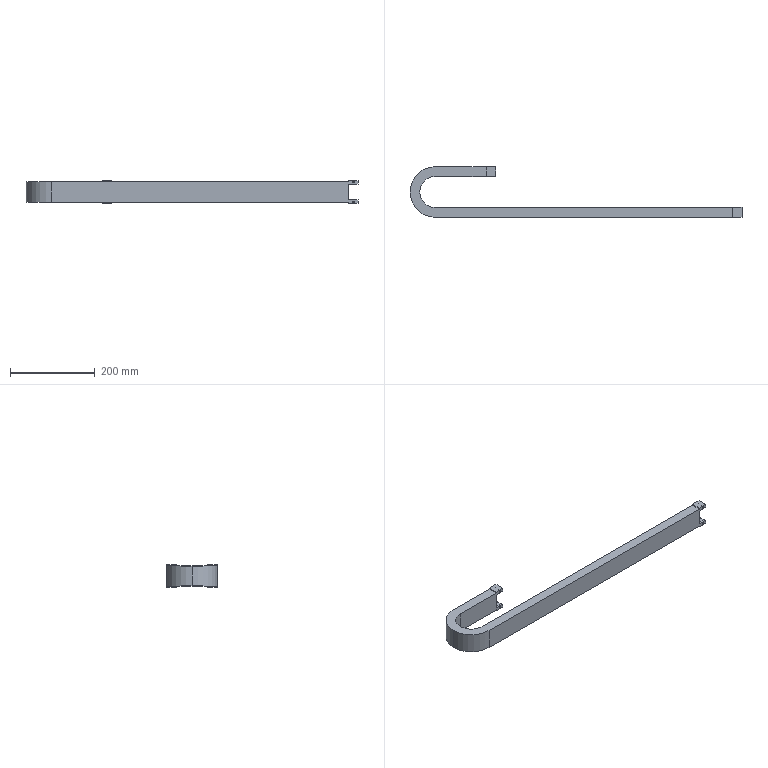Part | SolidWorks | features ICE 12, Fillet 2, HoleWzd 2, Shell 1, Sweep 1 | 1 solid | 72 faces | box 781.5 x 119 x 54 mm | volume 397201 mm3 | plane 56 | cylinder 16 | commonest cylinder face diameters 4.2 x8 73 x2 79 x2 113 x2 119 x2